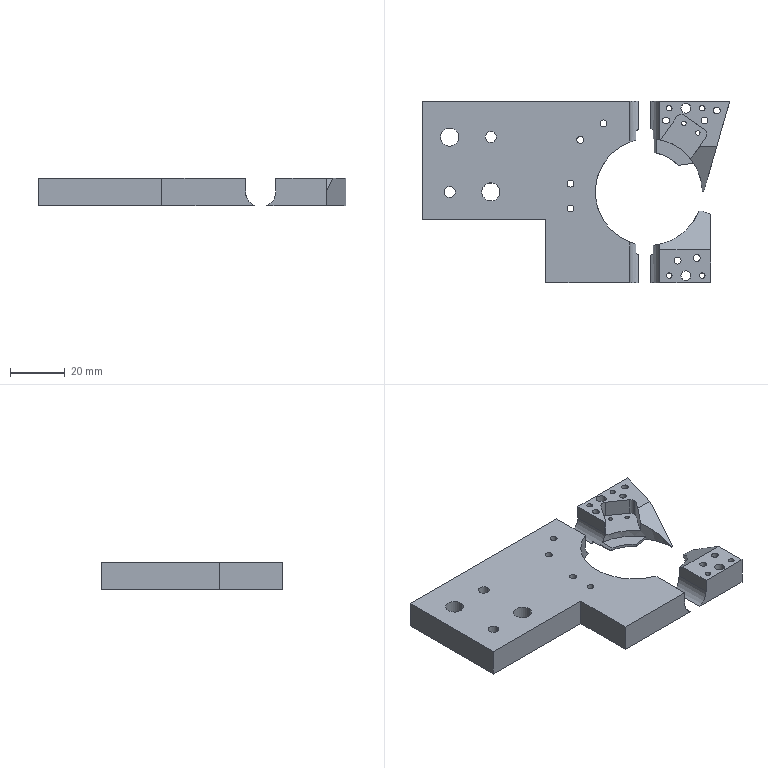Part | SolidWorks | features ICE 8, Extrusion 1 | 3 solids | 92 faces | box 112 x 66 x 10 mm | volume 41293 mm3 | cylinder 58 | plane 34 | commonest cylinder face diameters 2.5 x18 2 x8 4 x7 1.6 x4 3.6 x4 6.6 x4